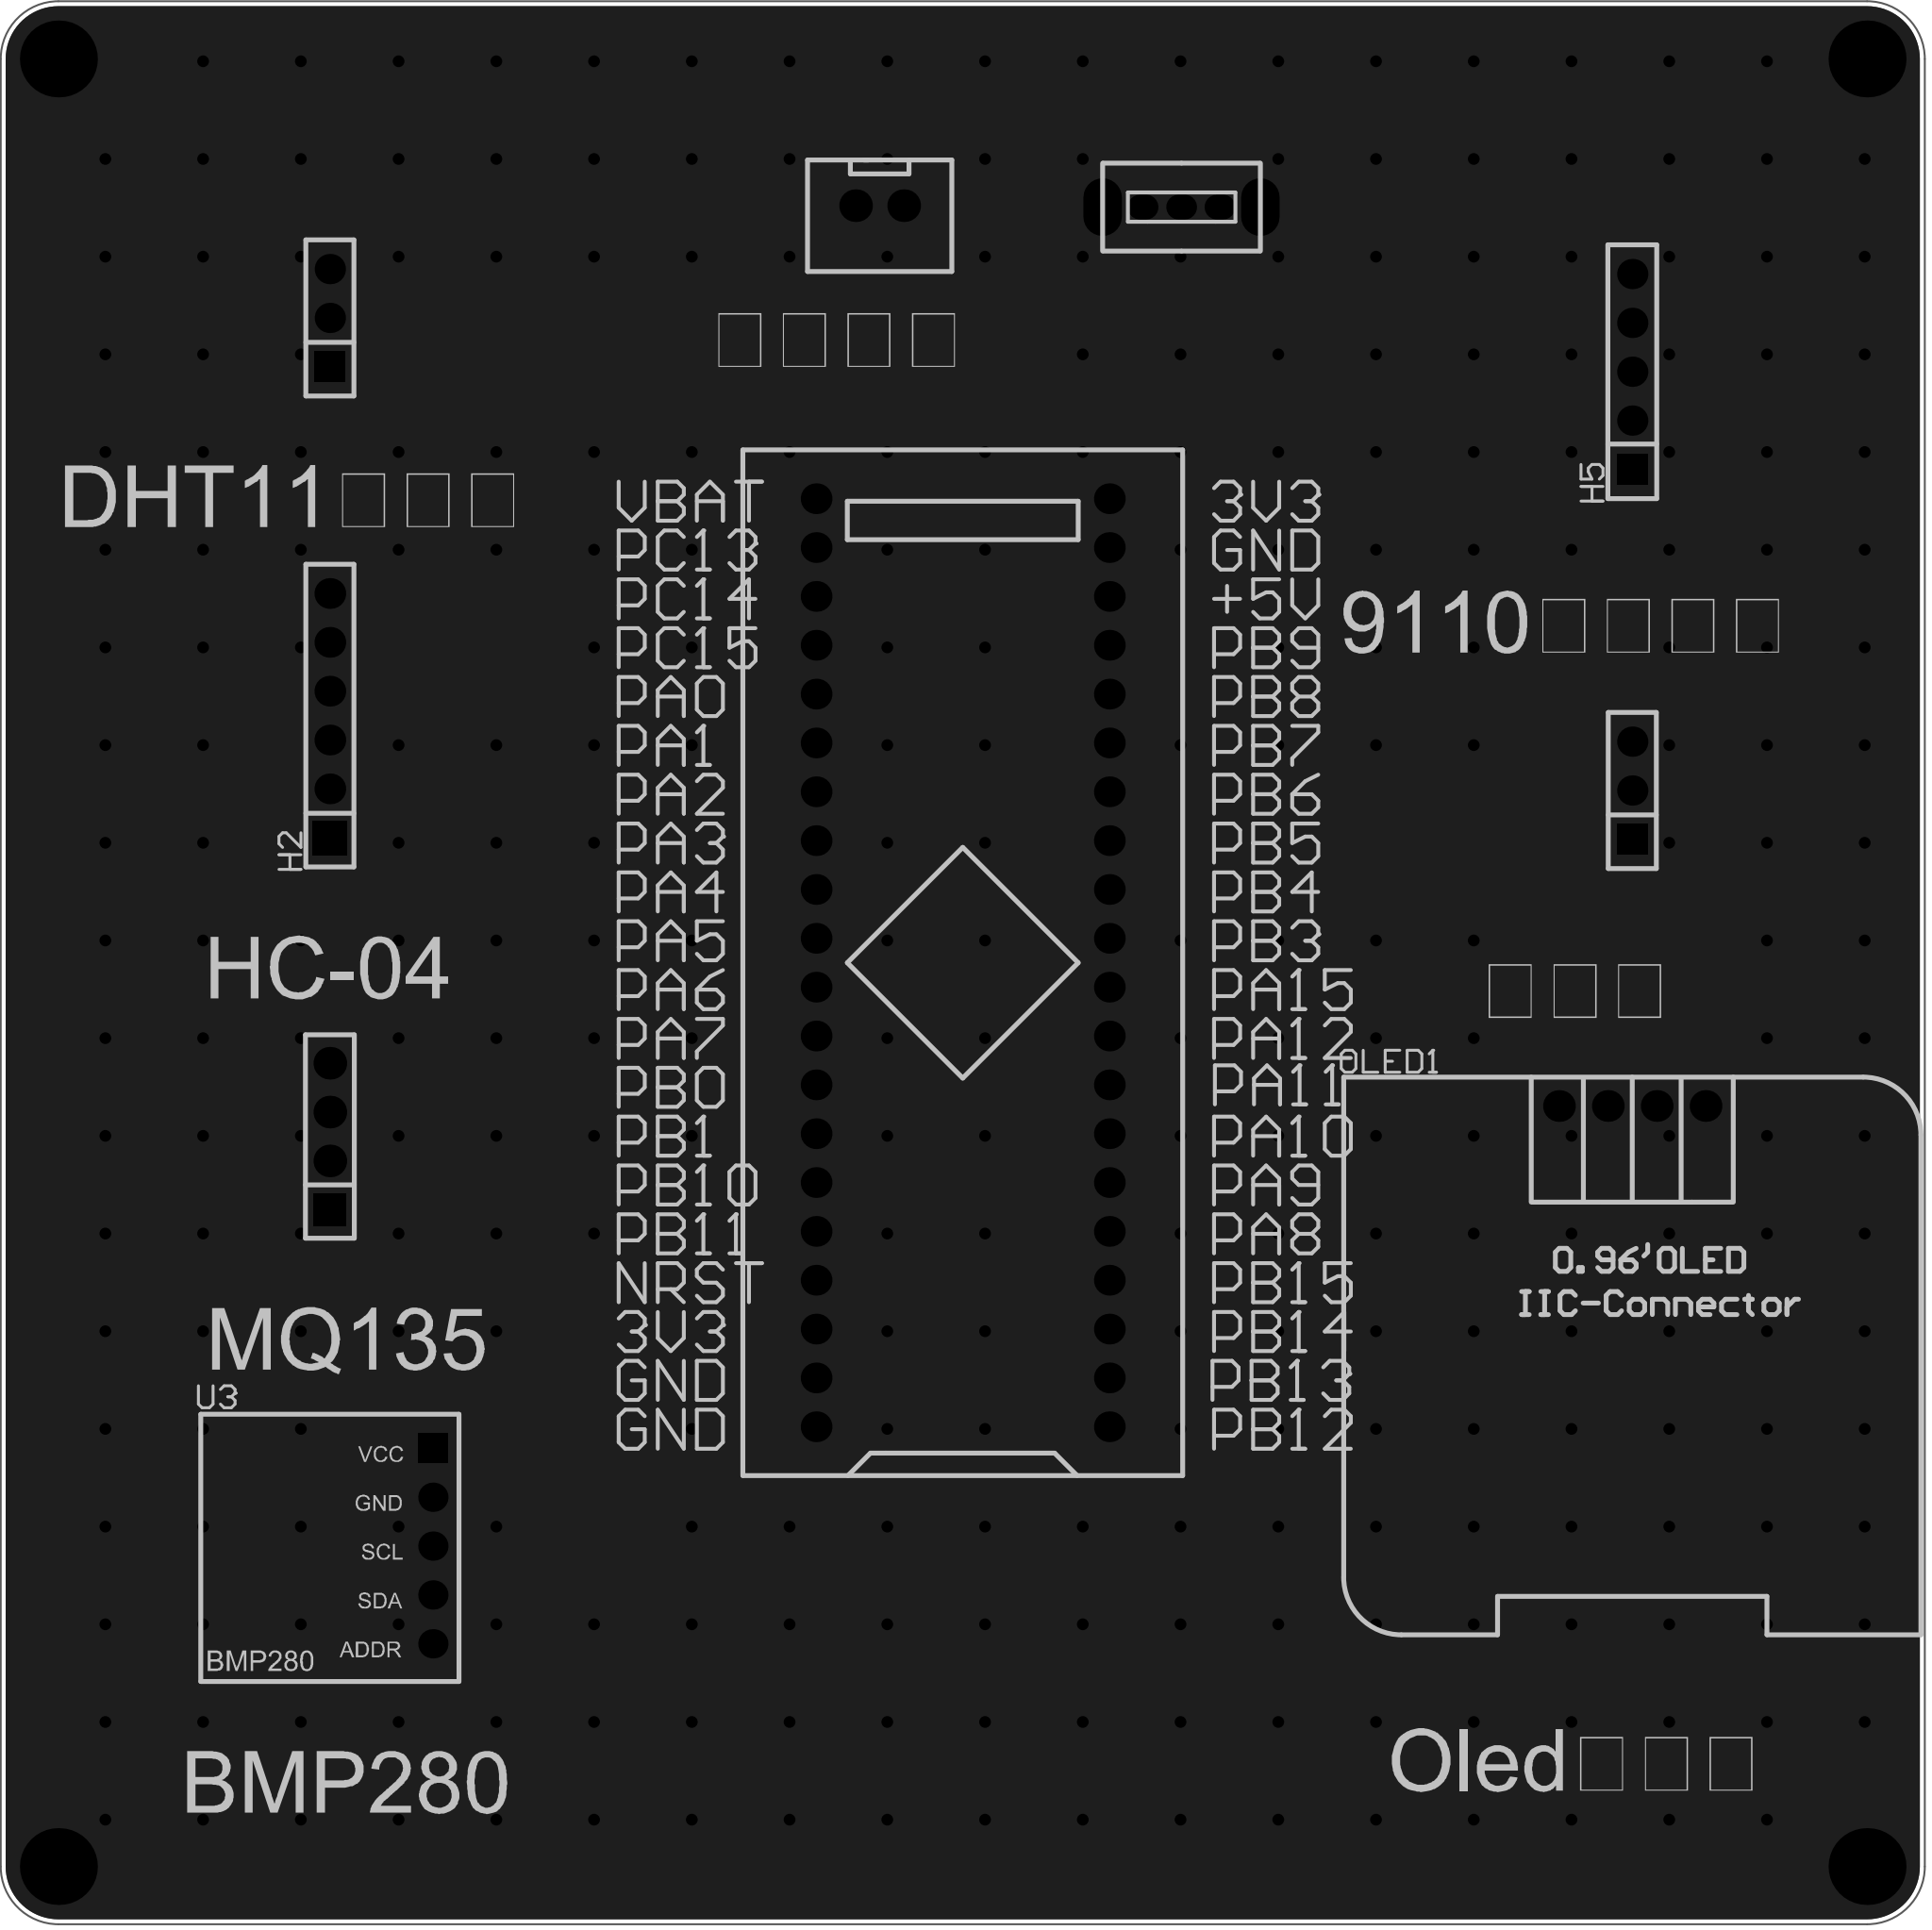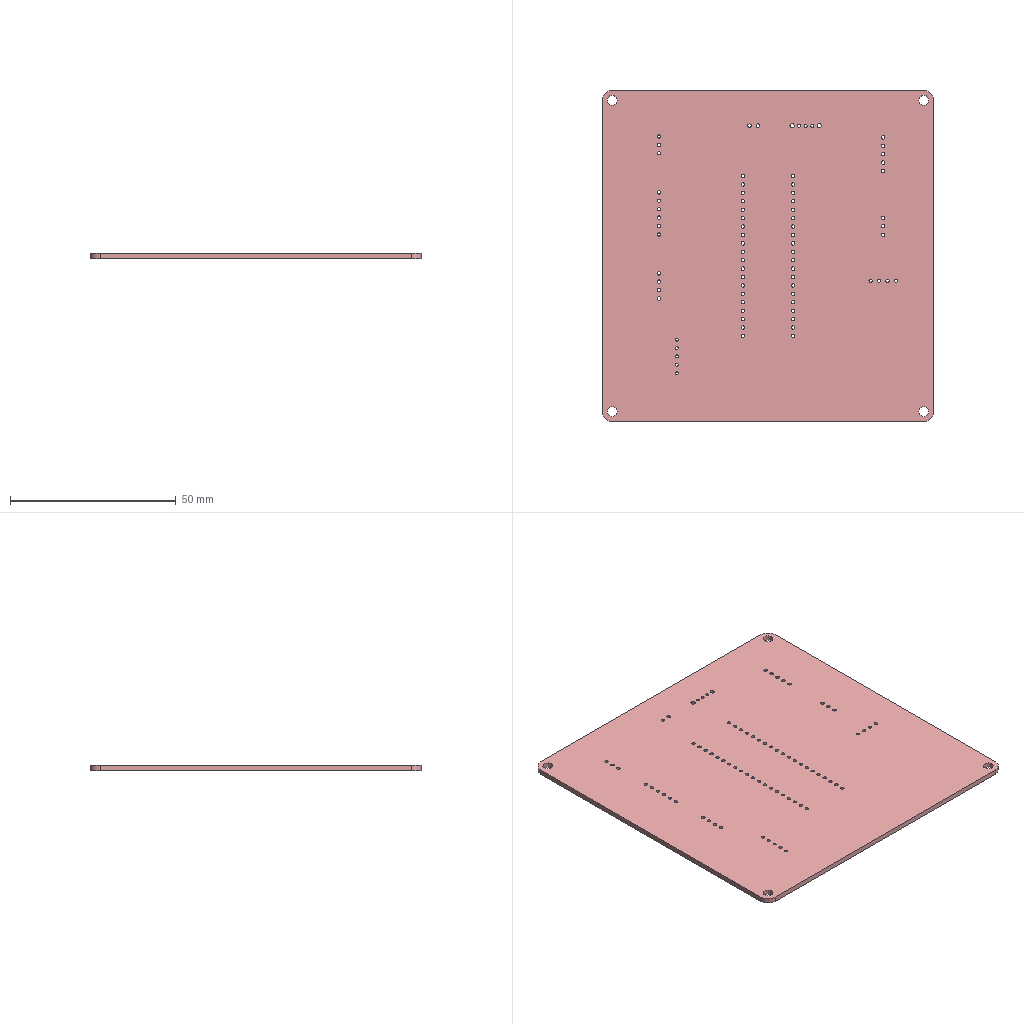Circuit board layout | Altium Designer | box 100 x 100 x 1.6 mm
Layer stack:
# Altium Designer layer stack of  (unit mm; dielectric type: 0 none, 1 core, 2 prepreg, 3 surface material)
index,name,kind,layer,copper_thickness_mm,dielectric_type,dielectric_thickness_mm,dielectric_material,dielectric_constant
0,Top Paste Mask Layer,other,,,,,,
1,Top Silkscreen Layer,other,,,,,,
2,Top Solder Mask Layer,dielectric,,,3,0.01,,3.3
3,Top Layer,copper,Top Layer,0.035,,,,
4,Dielectric1,dielectric,,,3,1.51,FR4,4.5
5,Bottom Layer,copper,Bottom Layer,0.035,,,,
6,Bottom Solder Mask Layer,dielectric,,,3,0.01,,3.3
7,Bottom Silkscreen Layer,other,,,,,,
8,Bottom Paste Mask Layer,other,,,,,,
# drill layer pairs: low layer,high layer
drill_pair,Top Layer,Bottom Layer
Part placement:
Designator,Comment,Layer,Footprint,Center-X(mm),Center-Y(mm),Rotation
U1,STM32F103C8T6-Card,TopLayer,CONN-TH_L53.3-W22.9_STM32F103C8T6-CARD,141.351,130.937,90
CN4,XH2.54*2P_直插,TopLayer,CONN-TH_2P-P2.50-XH2.54-2P,137.033,170.307,0
SW5,,TopLayer,拨动开关,152.72,170.232,180
H1,,TopLayer,HDR-TH_3P-P2.54-V-F,176.149,139.894,90
H3,,TopLayer,HDR-TH_3P-P2.54-V-F,108.458,164.469,90
H4,,TopLayer,HDR-TH_4P-P2.54-V-F,108.458,121.901,90
U3,,TopLayer,BH1750光照传感器,113.813,100.601,0
H2,,TopLayer,HDR-TH_6P-P2.54-V-F,108.458,143.789,90
H5,,TopLayer,HDR-TH_5P-P2.54-V-F,176.149,161.671,90
OLED1,,TopLayer,0.96OLED_4P,176.149,123.487,0
Pad and via stacks:
# Altium Designer via and pad stacks of  (unit mm). Each distinct definition once, with the count of objects using it.
# via: kind,start_layer,end_layer,hole_mm,diameter_mm,mode(0 simple;1 top-mid-bottom;2 full stack),diameter_per_layer,count,example_net
# pad: kind,layer,hole_mm,hole_type(0 round;1 square;2 slot),plating,top_size,top_shape(1 round;2 rect;3 octagon;9 rounded rect),mid_size,bottom_size,mode,footprint,size_per_layer,count,example
pad,Multi-Layer,3,0,plated,4x4,1,4x4,4x4,0,,,4,1
pad,Multi-Layer,1,0,plated,1.6x1.6,1,1.6x1.6,1.6x1.6,0,CONN-TH_L53.3-W22.9_STM32F103C8T6-CARD,,40,U1.1
pad,Multi-Layer,1.05,0,plated,1.7x1.7,1,1.7x1.7,1.7x1.7,0,CONN-TH_2P-P2.50-XH2.54-2P,,2,CN4.2
pad,Multi-Layer,0.8992,0,plated,1.6x1.3,1,1.6x1.3,1.6x1.3,0,\u00B2\u00A6\u00B6\u00AF\u00BF\u00AA\u00B9\u00D8,,3,SW5.1
pad,Multi-Layer,1.3,0,plated,3x1.999,1,3x1.999,3x1.999,0,\u00B2\u00A6\u00B6\u00AF\u00BF\u00AA\u00B9\u00D8,,2,SW5.4
pad,Multi-Layer,1.02,0,plated,1.575x1.575,1,1.575x1.575,1.575x1.575,0,HDR-TH_3P-P2.54-V-F,,4,H1.3
pad,Multi-Layer,1.02,0,plated,1.575x1.575,2,1.575x1.575,1.575x1.575,0,HDR-TH_3P-P2.54-V-F,,2,H1.1
pad,Multi-Layer,1.1,0,plated,1.7x1.7,2,1.7x1.7,1.7x1.7,0,HDR-TH_4P-P2.54-V-F,,1,H4.1
pad,Multi-Layer,1.1,0,plated,1.7x1.7,1,1.7x1.7,1.7x1.7,0,HDR-TH_4P-P2.54-V-F,,3,H4.2
pad,Multi-Layer,0.9144,0,plated,1.524x1.524,2,1.524x1.524,1.524x1.524,0,BH1750\u00B9\u00E2\u00D5\u00D5\u00B4\u00AB\u00B8\u00D0\u00C6\u00F7,,1,U3.1
pad,Multi-Layer,0.9144,0,plated,1.524x1.524,1,1.524x1.524,1.524x1.524,0,BH1750\u00B9\u00E2\u00D5\u00D5\u00B4\u00AB\u00B8\u00D0\u00C6\u00F7,,4,U3.4
pad,Multi-Layer,1.02,0,plated,1.6x1.6,1,1.6x1.6,1.6x1.6,0,HDR-TH_6P-P2.54-V-F,,5,H2.6
pad,Multi-Layer,1.02,0,plated,1.8x1.8,2,1.8x1.8,1.8x1.8,0,HDR-TH_6P-P2.54-V-F,,1,H2.1
pad,Multi-Layer,1.02,0,plated,1.575x1.575,1,1.575x1.575,1.575x1.575,0,HDR-TH_5P-P2.54-V-F,,4,H5.5
pad,Multi-Layer,1.02,0,plated,1.575x1.575,2,1.575x1.575,1.575x1.575,0,HDR-TH_5P-P2.54-V-F,,1,H5.1
pad,Multi-Layer,1,0,plated,1.65x1.65,1,1.65x1.65,1.65x1.65,0,0.96OLED_4P,,4,OLED1.4
via,Top Layer,Bottom Layer,0.3048,0.61,0,,306,GND
Copper pours:
name,layer,net,type(0 solid;1 hatched;2 none)
Bottom Layer-GND,Bottom Layer,GND,0
Top Layer-GND,Top Layer,GND,0
Design rules, without the lines most boards share:
# Altium Designer design rules of  (exported by Altium Designer, unit mm)
# columns: name | kind | enabled | priority | scope1 | scope2 | descriptor | typed fields (field=value)
Copper_copperRegion_copperThickness1oz | 0 | disabled | 4 | All | All | Clearance Constraint (Gap=5.984mil) (Disabled)(All),(All) | gap=0.152
Copper_copperRegion_copperThickness1oz_1 | 63 | disabled | 4 | All | All | Board Clearance Constraint (Gap=0mil) (Disabled)(All) |
Copper_copperRegion_Copper_copperRegion | 0 | disabled | 5 | All | All | Clearance Constraint (Gap=5.984mil) (Disabled)(All),(All) | gap=0.152
Copper_copperRegion_Copper_copperRegion_1 | 63 | disabled | 5 | All | All | Board Clearance Constraint (Gap=0mil) (Disabled)(All) |
copperThickness1oz | 0 | enabled | 6 | All | All | Clearance Constraint (Gap=5.984mil) (All),(All) | gap=0.152
copperThickness1oz_1 | 63 | enabled | 6 | All | All | Board Clearance Constraint (Gap=0mil) (All) |
copperRegion_copperThickness1oz | 20 | disabled | 1 | All | All | Polygon Connect Rule(Relief Connect )(Conductor Width=10mil) (Relief Angle=90 Angle) (Entries=4) (Air Gap Width=10mil) (Disabled)(All),(All) | connect_style(0=relief,1=direct,2=none)=0 relief_conductor_width=0.254 relief_entries=4
copperRegion_Copper_copperRegion | 20 | disabled | 2 | All | All | Polygon Connect Rule(Relief Connect )(Conductor Width=10mil) (Relief Angle=90 Angle) (Entries=4) (Air Gap Width=10mil) (Disabled)(All),(All) | connect_style(0=relief,1=direct,2=none)=0 relief_conductor_width=0.254 relief_entries=4
copperRegion | 20 | enabled | 3 | All | All | Polygon Connect Rule(Relief Connect )(Conductor Width=10mil) (Relief Angle=90 Angle) (Entries=4) (Air Gap Width=10mil) (All),(All) | connect_style(0=relief,1=direct,2=none)=0 relief_conductor_width=0.254 relief_entries=4